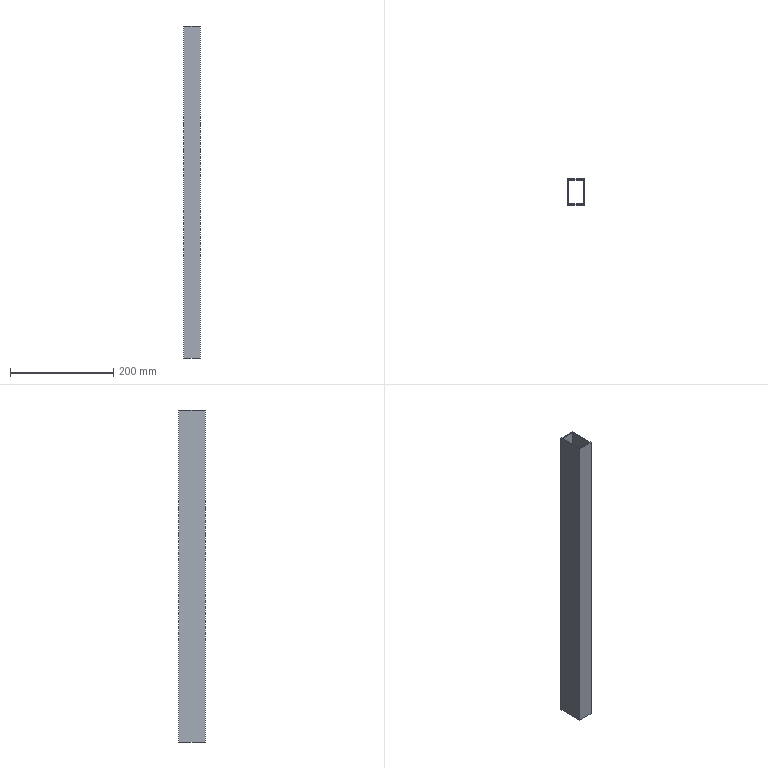Part | SolidWorks | features Extrusion 1 | 1 solid | 10 faces | box 31.516 x 51.109 x 644 mm | volume 202538 mm3 | plane 10
STEP:
#1=CARTESIAN_POINT('',(-80.505,-24.284,644.));
#2=VERTEX_POINT('',#1);
#3=CARTESIAN_POINT('',(-48.989,-24.284,644.));
#4=VERTEX_POINT('',#3);
#5=CARTESIAN_POINT('',(-48.989,-24.284,644.));
#6=DIRECTION('',(1.,0.,0.));
#7=VECTOR('',#6,1000.);
#8=LINE('',#5,#7);
#9=EDGE_CURVE('',#2,#4,#8,.T.);
#10=ORIENTED_EDGE('',*,*,#9,.F.);
#11=CARTESIAN_POINT('',(-80.505,-24.284,0.));
#12=VERTEX_POINT('',#11);
#13=CARTESIAN_POINT('',(-80.505,-24.284,704.045));
#14=DIRECTION('',(0.,0.,-1.));
#15=VECTOR('',#14,1000.);
#16=LINE('',#13,#15);
#17=EDGE_CURVE('',#2,#12,#16,.T.);
#18=ORIENTED_EDGE('',*,*,#17,.T.);
#19=CARTESIAN_POINT('',(-48.989,-24.284,0.));
#20=VERTEX_POINT('',#19);
#21=CARTESIAN_POINT('',(-48.989,-24.284,0.));
#22=DIRECTION('',(1.,0.,0.));
#23=VECTOR('',#22,1000.);
#24=LINE('',#21,#23);
#25=EDGE_CURVE('',#12,#20,#24,.T.);
#26=ORIENTED_EDGE('',*,*,#25,.T.);
#27=CARTESIAN_POINT('',(-48.989,-24.284,704.045));
#28=DIRECTION('',(0.,0.,-1.));
#29=VECTOR('',#28,1000.);
#30=LINE('',#27,#29);
#31=EDGE_CURVE('',#4,#20,#30,.T.);
#32=ORIENTED_EDGE('',*,*,#31,.F.);
#33=EDGE_LOOP('',(#10,#18,#26,#32));
#34=FACE_OUTER_BOUND('',#33,.T.);
#35=CARTESIAN_POINT('',(-48.989,-24.284,704.045));
#36=DIRECTION('',(0.,1.,0.));
#37=DIRECTION('',(-1.,0.,0.));
#38=AXIS2_PLACEMENT_3D('',#35,#36,#37);
#39=PLANE('',#38);
#40=ADVANCED_FACE('',(#34),#39,.F.);
#41=CARTESIAN_POINT('',(-80.505,26.825,644.));
#42=VERTEX_POINT('',#41);
#43=CARTESIAN_POINT('',(-80.505,26.825,644.));
#44=DIRECTION('',(0.,-1.,0.));
#45=VECTOR('',#44,1000.);
#46=LINE('',#43,#45);
#47=EDGE_CURVE('',#42,#2,#46,.T.);
#48=ORIENTED_EDGE('',*,*,#47,.F.);
#49=CARTESIAN_POINT('',(-80.505,26.825,0.));
#50=VERTEX_POINT('',#49);
#51=CARTESIAN_POINT('',(-80.505,26.825,704.045));
#52=DIRECTION('',(0.,0.,-1.));
#53=VECTOR('',#52,1000.);
#54=LINE('',#51,#53);
#55=EDGE_CURVE('',#42,#50,#54,.T.);
#56=ORIENTED_EDGE('',*,*,#55,.T.);
#57=CARTESIAN_POINT('',(-80.505,26.825,0.));
#58=DIRECTION('',(0.,-1.,0.));
#59=VECTOR('',#58,1000.);
#60=LINE('',#57,#59);
#61=EDGE_CURVE('',#50,#12,#60,.T.);
#62=ORIENTED_EDGE('',*,*,#61,.T.);
#63=ORIENTED_EDGE('',*,*,#17,.F.);
#64=EDGE_LOOP('',(#48,#56,#62,#63));
#65=FACE_OUTER_BOUND('',#64,.T.);
#66=CARTESIAN_POINT('',(-80.505,26.825,704.045));
#67=DIRECTION('',(1.,0.,0.));
#68=DIRECTION('',(0.,0.,-1.));
#69=AXIS2_PLACEMENT_3D('',#66,#67,#68);
#70=PLANE('',#69);
#71=ADVANCED_FACE('',(#65),#70,.F.);
#72=CARTESIAN_POINT('',(-48.989,26.825,644.));
#73=VERTEX_POINT('',#72);
#74=CARTESIAN_POINT('',(-48.989,26.825,644.));
#75=DIRECTION('',(-1.,0.,0.));
#76=VECTOR('',#75,1000.);
#77=LINE('',#74,#76);
#78=EDGE_CURVE('',#73,#42,#77,.T.);
#79=ORIENTED_EDGE('',*,*,#78,.F.);
#80=CARTESIAN_POINT('',(-48.989,26.825,0.));
#81=VERTEX_POINT('',#80);
#82=CARTESIAN_POINT('',(-48.989,26.825,704.045));
#83=DIRECTION('',(0.,0.,-1.));
#84=VECTOR('',#83,1000.);
#85=LINE('',#82,#84);
#86=EDGE_CURVE('',#73,#81,#85,.T.);
#87=ORIENTED_EDGE('',*,*,#86,.T.);
#88=CARTESIAN_POINT('',(-48.989,26.825,0.));
#89=DIRECTION('',(-1.,0.,0.));
#90=VECTOR('',#89,1000.);
#91=LINE('',#88,#90);
#92=EDGE_CURVE('',#81,#50,#91,.T.);
#93=ORIENTED_EDGE('',*,*,#92,.T.);
#94=ORIENTED_EDGE('',*,*,#55,.F.);
#95=EDGE_LOOP('',(#79,#87,#93,#94));
#96=FACE_OUTER_BOUND('',#95,.T.);
#97=CARTESIAN_POINT('',(-48.989,26.825,704.045));
#98=DIRECTION('',(0.,-1.,0.));
#99=DIRECTION('',(0.,0.,-1.));
#100=AXIS2_PLACEMENT_3D('',#97,#98,#99);
#101=PLANE('',#100);
#102=ADVANCED_FACE('',(#96),#101,.F.);
#103=CARTESIAN_POINT('',(-48.989,26.825,644.));
#104=DIRECTION('',(0.,1.,0.));
#105=VECTOR('',#104,1000.);
#106=LINE('',#103,#105);
#107=EDGE_CURVE('',#4,#73,#106,.T.);
#108=ORIENTED_EDGE('',*,*,#107,.F.);
#109=ORIENTED_EDGE('',*,*,#31,.T.);
#110=CARTESIAN_POINT('',(-48.989,26.825,0.));
#111=DIRECTION('',(0.,1.,0.));
#112=VECTOR('',#111,1000.);
#113=LINE('',#110,#112);
#114=EDGE_CURVE('',#20,#81,#113,.T.);
#115=ORIENTED_EDGE('',*,*,#114,.T.);
#116=ORIENTED_EDGE('',*,*,#86,.F.);
#117=EDGE_LOOP('',(#108,#109,#115,#116));
#118=FACE_OUTER_BOUND('',#117,.T.);
#119=CARTESIAN_POINT('',(-48.989,26.825,704.045));
#120=DIRECTION('',(-1.,0.,0.));
#121=DIRECTION('',(0.,0.,1.));
#122=AXIS2_PLACEMENT_3D('',#119,#120,#121);
#123=PLANE('',#122);
#124=ADVANCED_FACE('',(#118),#123,.F.);
#125=ORIENTED_EDGE('',*,*,#114,.F.);
#126=ORIENTED_EDGE('',*,*,#25,.F.);
#127=ORIENTED_EDGE('',*,*,#61,.F.);
#128=ORIENTED_EDGE('',*,*,#92,.F.);
#129=EDGE_LOOP('',(#125,#126,#127,#128));
#130=FACE_OUTER_BOUND('',#129,.T.);
#131=CARTESIAN_POINT('',(-78.505,-22.284,0.));
#132=VERTEX_POINT('',#131);
#133=CARTESIAN_POINT('',(-50.989,-22.284,0.));
#134=VERTEX_POINT('',#133);
#135=CARTESIAN_POINT('',(-50.989,-22.284,0.));
#136=DIRECTION('',(1.,0.,0.));
#137=VECTOR('',#136,1000.);
#138=LINE('',#135,#137);
#139=EDGE_CURVE('',#132,#134,#138,.T.);
#140=ORIENTED_EDGE('',*,*,#139,.T.);
#141=CARTESIAN_POINT('',(-50.989,24.825,0.));
#142=VERTEX_POINT('',#141);
#143=CARTESIAN_POINT('',(-50.989,24.825,0.));
#144=DIRECTION('',(0.,1.,0.));
#145=VECTOR('',#144,1000.);
#146=LINE('',#143,#145);
#147=EDGE_CURVE('',#134,#142,#146,.T.);
#148=ORIENTED_EDGE('',*,*,#147,.T.);
#149=CARTESIAN_POINT('',(-78.505,24.825,0.));
#150=VERTEX_POINT('',#149);
#151=CARTESIAN_POINT('',(-50.989,24.825,0.));
#152=DIRECTION('',(-1.,0.,0.));
#153=VECTOR('',#152,1000.);
#154=LINE('',#151,#153);
#155=EDGE_CURVE('',#142,#150,#154,.T.);
#156=ORIENTED_EDGE('',*,*,#155,.T.);
#157=CARTESIAN_POINT('',(-78.505,24.825,0.));
#158=DIRECTION('',(0.,-1.,0.));
#159=VECTOR('',#158,1000.);
#160=LINE('',#157,#159);
#161=EDGE_CURVE('',#150,#132,#160,.T.);
#162=ORIENTED_EDGE('',*,*,#161,.T.);
#163=EDGE_LOOP('',(#140,#148,#156,#162));
#164=FACE_BOUND('',#163,.T.);
#165=CARTESIAN_POINT('',(0.,0.,0.));
#166=DIRECTION('',(0.,0.,-1.));
#167=DIRECTION('',(-1.,0.,0.));
#168=AXIS2_PLACEMENT_3D('',#165,#166,#167);
#169=PLANE('',#168);
#170=ADVANCED_FACE('',(#130,#164),#169,.T.);
#171=CARTESIAN_POINT('',(-78.505,-22.284,644.));
#172=VERTEX_POINT('',#171);
#173=CARTESIAN_POINT('',(-78.505,-22.284,704.045));
#174=DIRECTION('',(0.,0.,-1.));
#175=VECTOR('',#174,1000.);
#176=LINE('',#173,#175);
#177=EDGE_CURVE('',#172,#132,#176,.T.);
#178=ORIENTED_EDGE('',*,*,#177,.F.);
#179=CARTESIAN_POINT('',(-50.989,-22.284,644.));
#180=VERTEX_POINT('',#179);
#181=CARTESIAN_POINT('',(-50.989,-22.284,644.));
#182=DIRECTION('',(1.,0.,0.));
#183=VECTOR('',#182,1000.);
#184=LINE('',#181,#183);
#185=EDGE_CURVE('',#172,#180,#184,.T.);
#186=ORIENTED_EDGE('',*,*,#185,.T.);
#187=CARTESIAN_POINT('',(-50.989,-22.284,704.045));
#188=DIRECTION('',(0.,0.,-1.));
#189=VECTOR('',#188,1000.);
#190=LINE('',#187,#189);
#191=EDGE_CURVE('',#180,#134,#190,.T.);
#192=ORIENTED_EDGE('',*,*,#191,.T.);
#193=ORIENTED_EDGE('',*,*,#139,.F.);
#194=EDGE_LOOP('',(#178,#186,#192,#193));
#195=FACE_OUTER_BOUND('',#194,.T.);
#196=CARTESIAN_POINT('',(-50.989,-22.284,704.045));
#197=DIRECTION('',(0.,1.,0.));
#198=DIRECTION('',(0.,0.,1.));
#199=AXIS2_PLACEMENT_3D('',#196,#197,#198);
#200=PLANE('',#199);
#201=ADVANCED_FACE('',(#195),#200,.T.);
#202=CARTESIAN_POINT('',(-78.505,24.825,644.));
#203=VERTEX_POINT('',#202);
#204=CARTESIAN_POINT('',(-78.505,24.825,704.045));
#205=DIRECTION('',(0.,0.,-1.));
#206=VECTOR('',#205,1000.);
#207=LINE('',#204,#206);
#208=EDGE_CURVE('',#203,#150,#207,.T.);
#209=ORIENTED_EDGE('',*,*,#208,.F.);
#210=CARTESIAN_POINT('',(-78.505,24.825,644.));
#211=DIRECTION('',(0.,-1.,0.));
#212=VECTOR('',#211,1000.);
#213=LINE('',#210,#212);
#214=EDGE_CURVE('',#203,#172,#213,.T.);
#215=ORIENTED_EDGE('',*,*,#214,.T.);
#216=ORIENTED_EDGE('',*,*,#177,.T.);
#217=ORIENTED_EDGE('',*,*,#161,.F.);
#218=EDGE_LOOP('',(#209,#215,#216,#217));
#219=FACE_OUTER_BOUND('',#218,.T.);
#220=CARTESIAN_POINT('',(-78.505,24.825,704.045));
#221=DIRECTION('',(1.,0.,0.));
#222=DIRECTION('',(0.,0.,-1.));
#223=AXIS2_PLACEMENT_3D('',#220,#221,#222);
#224=PLANE('',#223);
#225=ADVANCED_FACE('',(#219),#224,.T.);
#226=CARTESIAN_POINT('',(-50.989,24.825,644.));
#227=VERTEX_POINT('',#226);
#228=CARTESIAN_POINT('',(-50.989,24.825,704.045));
#229=DIRECTION('',(0.,0.,-1.));
#230=VECTOR('',#229,1000.);
#231=LINE('',#228,#230);
#232=EDGE_CURVE('',#227,#142,#231,.T.);
#233=ORIENTED_EDGE('',*,*,#232,.F.);
#234=CARTESIAN_POINT('',(-50.989,24.825,644.));
#235=DIRECTION('',(-1.,0.,0.));
#236=VECTOR('',#235,1000.);
#237=LINE('',#234,#236);
#238=EDGE_CURVE('',#227,#203,#237,.T.);
#239=ORIENTED_EDGE('',*,*,#238,.T.);
#240=ORIENTED_EDGE('',*,*,#208,.T.);
#241=ORIENTED_EDGE('',*,*,#155,.F.);
#242=EDGE_LOOP('',(#233,#239,#240,#241));
#243=FACE_OUTER_BOUND('',#242,.T.);
#244=CARTESIAN_POINT('',(-50.989,24.825,704.045));
#245=DIRECTION('',(0.,-1.,0.));
#246=DIRECTION('',(0.,0.,-1.));
#247=AXIS2_PLACEMENT_3D('',#244,#245,#246);
#248=PLANE('',#247);
#249=ADVANCED_FACE('',(#243),#248,.T.);
#250=ORIENTED_EDGE('',*,*,#191,.F.);
#251=CARTESIAN_POINT('',(-50.989,24.825,644.));
#252=DIRECTION('',(0.,1.,0.));
#253=VECTOR('',#252,1000.);
#254=LINE('',#251,#253);
#255=EDGE_CURVE('',#180,#227,#254,.T.);
#256=ORIENTED_EDGE('',*,*,#255,.T.);
#257=ORIENTED_EDGE('',*,*,#232,.T.);
#258=ORIENTED_EDGE('',*,*,#147,.F.);
#259=EDGE_LOOP('',(#250,#256,#257,#258));
#260=FACE_OUTER_BOUND('',#259,.T.);
#261=CARTESIAN_POINT('',(-50.989,24.825,704.045));
#262=DIRECTION('',(-1.,0.,0.));
#263=DIRECTION('',(0.,0.,1.));
#264=AXIS2_PLACEMENT_3D('',#261,#262,#263);
#265=PLANE('',#264);
#266=ADVANCED_FACE('',(#260),#265,.T.);
#267=ORIENTED_EDGE('',*,*,#185,.F.);
#268=ORIENTED_EDGE('',*,*,#214,.F.);
#269=ORIENTED_EDGE('',*,*,#238,.F.);
#270=ORIENTED_EDGE('',*,*,#255,.F.);
#271=EDGE_LOOP('',(#267,#268,#269,#270));
#272=FACE_BOUND('',#271,.T.);
#273=ORIENTED_EDGE('',*,*,#107,.T.);
#274=ORIENTED_EDGE('',*,*,#78,.T.);
#275=ORIENTED_EDGE('',*,*,#47,.T.);
#276=ORIENTED_EDGE('',*,*,#9,.T.);
#277=EDGE_LOOP('',(#273,#274,#275,#276));
#278=FACE_OUTER_BOUND('',#277,.T.);
#279=CARTESIAN_POINT('',(0.,0.,644.));
#280=DIRECTION('',(0.,0.,1.));
#281=DIRECTION('',(1.,0.,0.));
#282=AXIS2_PLACEMENT_3D('',#279,#280,#281);
#283=PLANE('',#282);
#284=ADVANCED_FACE('',(#272,#278),#283,.T.);
#285=CLOSED_SHELL('',(#40,#71,#102,#124,#170,#201,#225,#249,#266,#284));
#286=MANIFOLD_SOLID_BREP('',#285);
#287=CARTESIAN_POINT('',(0.,0.,0.));
#288=DIRECTION('',(0.,0.,1.));
#289=DIRECTION('',(1.,0.,0.));
#290=AXIS2_PLACEMENT_3D('',#287,#288,#289);
#291=(LENGTH_UNIT()NAMED_UNIT(*)SI_UNIT(.MILLI.,.METRE.));
#292=UNCERTAINTY_MEASURE_WITH_UNIT(LENGTH_MEASURE(0.00001),#291,'','');
#293=(NAMED_UNIT(*)PLANE_ANGLE_UNIT()SI_UNIT($,.RADIAN.));
#294=(NAMED_UNIT(*)SI_UNIT($,.STERADIAN.)SOLID_ANGLE_UNIT());
#295=(GEOMETRIC_REPRESENTATION_CONTEXT(3)GLOBAL_UNCERTAINTY_ASSIGNED_CONTEXT((#292))GLOBAL_UNIT_ASSIGNED_CONTEXT((#291,#293,#294))REPRESENTATION_CONTEXT('',''));
#296=ADVANCED_BREP_SHAPE_REPRESENTATION('',(#286,#290),#295);